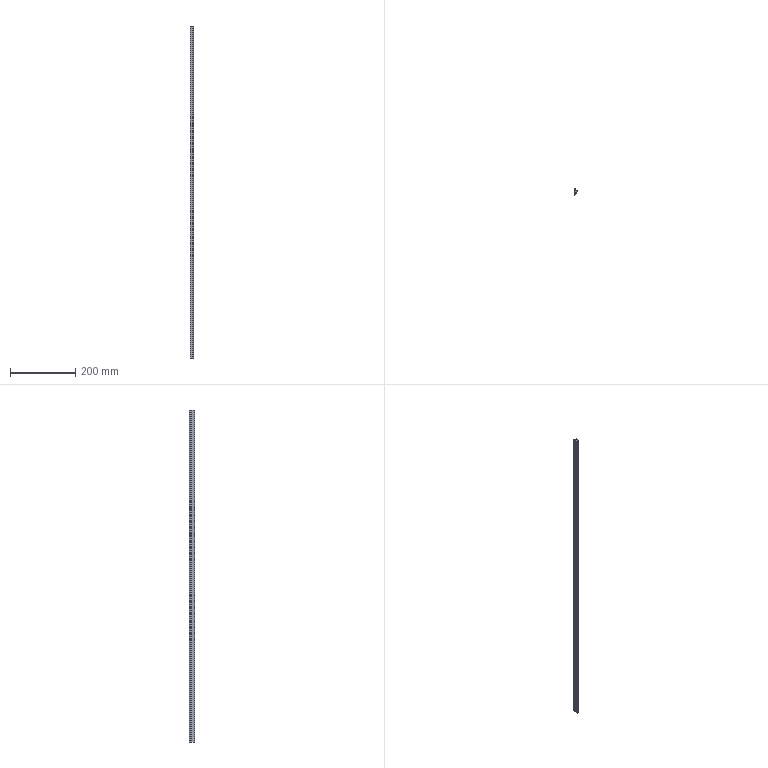Part | SolidWorks | features BaseBody 1, MoveFace 1 | 1 solid | 20 faces | box 10.8 x 17.5 x 1020 mm | volume 80377 mm3 | cylinder 11 | plane 9 | commonest cylinder face diameters 1.6 x2 14 x2 0.4 x1 0.6 x1 0.8 x1 2.6 x1
STEP:
#1=CARTESIAN_POINT('',(-3.236,-11.055,920.));
#2=VERTEX_POINT('',#1);
#3=CARTESIAN_POINT('',(-4.3,-10.3,920.));
#4=VERTEX_POINT('',#3);
#5=CARTESIAN_POINT('',(-3.5,-10.3,920.));
#6=DIRECTION('',(0.,0.,-1.));
#7=DIRECTION('',(1.,0.,0.));
#8=AXIS2_PLACEMENT_3D('',#5,#6,#7);
#9=CIRCLE('',#8,0.8);
#10=EDGE_CURVE('',#2,#4,#9,.T.);
#11=ORIENTED_EDGE('',*,*,#10,.T.);
#12=CARTESIAN_POINT('',(-4.3,-10.3,-100.));
#13=VERTEX_POINT('',#12);
#14=CARTESIAN_POINT('',(-4.3,-10.3,-100.));
#15=DIRECTION('',(0.,0.,-1.));
#16=VECTOR('',#15,1000.);
#17=LINE('',#14,#16);
#18=EDGE_CURVE('',#4,#13,#17,.T.);
#19=ORIENTED_EDGE('',*,*,#18,.T.);
#20=CARTESIAN_POINT('',(-3.236,-11.055,-100.));
#21=VERTEX_POINT('',#20);
#22=CARTESIAN_POINT('',(-3.5,-10.3,-100.));
#23=DIRECTION('',(0.,0.,1.));
#24=DIRECTION('',(-1.,0.,0.));
#25=AXIS2_PLACEMENT_3D('',#22,#23,#24);
#26=CIRCLE('',#25,0.8);
#27=EDGE_CURVE('',#13,#21,#26,.T.);
#28=ORIENTED_EDGE('',*,*,#27,.T.);
#29=CARTESIAN_POINT('',(-3.236,-11.055,-100.));
#30=DIRECTION('',(0.,0.,-1.));
#31=VECTOR('',#30,1000.);
#32=LINE('',#29,#31);
#33=EDGE_CURVE('',#2,#21,#32,.T.);
#34=ORIENTED_EDGE('',*,*,#33,.F.);
#35=EDGE_LOOP('',(#11,#19,#28,#34));
#36=FACE_OUTER_BOUND('',#35,.T.);
#37=CARTESIAN_POINT('',(-3.5,-10.3,-100.));
#38=DIRECTION('',(0.,0.,-1.));
#39=DIRECTION('',(-1.,0.,0.));
#40=AXIS2_PLACEMENT_3D('',#37,#38,#39);
#41=CYLINDRICAL_SURFACE('',#40,0.8);
#42=ADVANCED_FACE('',(#36),#41,.T.);
#43=CARTESIAN_POINT('',(1.184,-6.397,-100.));
#44=VERTEX_POINT('',#43);
#45=CARTESIAN_POINT('',(-5.702,-4.29,-100.));
#46=DIRECTION('',(0.,0.,1.));
#47=DIRECTION('',(-1.,0.,0.));
#48=AXIS2_PLACEMENT_3D('',#45,#46,#47);
#49=CIRCLE('',#48,7.201);
#50=EDGE_CURVE('',#21,#44,#49,.T.);
#51=ORIENTED_EDGE('',*,*,#50,.T.);
#52=CARTESIAN_POINT('',(1.184,-6.397,920.));
#53=VERTEX_POINT('',#52);
#54=CARTESIAN_POINT('',(1.184,-6.397,-100.));
#55=DIRECTION('',(0.,0.,1.));
#56=VECTOR('',#55,1000.);
#57=LINE('',#54,#56);
#58=EDGE_CURVE('',#44,#53,#57,.T.);
#59=ORIENTED_EDGE('',*,*,#58,.T.);
#60=CARTESIAN_POINT('',(-5.702,-4.29,920.));
#61=DIRECTION('',(0.,0.,-1.));
#62=DIRECTION('',(1.,0.,0.));
#63=AXIS2_PLACEMENT_3D('',#60,#61,#62);
#64=CIRCLE('',#63,7.201);
#65=EDGE_CURVE('',#53,#2,#64,.T.);
#66=ORIENTED_EDGE('',*,*,#65,.T.);
#67=ORIENTED_EDGE('',*,*,#33,.T.);
#68=EDGE_LOOP('',(#51,#59,#66,#67));
#69=FACE_OUTER_BOUND('',#68,.T.);
#70=CARTESIAN_POINT('',(-5.702,-4.29,-100.));
#71=DIRECTION('',(0.,0.,-1.));
#72=DIRECTION('',(-1.,0.,0.));
#73=AXIS2_PLACEMENT_3D('',#70,#71,#72);
#74=CYLINDRICAL_SURFACE('',#73,7.201);
#75=ADVANCED_FACE('',(#69),#74,.T.);
#76=CARTESIAN_POINT('',(0.9,-6.,-100.));
#77=VERTEX_POINT('',#76);
#78=CARTESIAN_POINT('',(0.9,-6.3,-100.));
#79=DIRECTION('',(0.,0.,1.));
#80=DIRECTION('',(-1.,0.,0.));
#81=AXIS2_PLACEMENT_3D('',#78,#79,#80);
#82=CIRCLE('',#81,0.3);
#83=EDGE_CURVE('',#44,#77,#82,.T.);
#84=ORIENTED_EDGE('',*,*,#83,.T.);
#85=CARTESIAN_POINT('',(0.9,-6.,920.));
#86=VERTEX_POINT('',#85);
#87=CARTESIAN_POINT('',(0.9,-6.,-100.));
#88=DIRECTION('',(0.,0.,1.));
#89=VECTOR('',#88,1000.);
#90=LINE('',#87,#89);
#91=EDGE_CURVE('',#77,#86,#90,.T.);
#92=ORIENTED_EDGE('',*,*,#91,.T.);
#93=CARTESIAN_POINT('',(0.9,-6.3,920.));
#94=DIRECTION('',(0.,0.,-1.));
#95=DIRECTION('',(1.,0.,0.));
#96=AXIS2_PLACEMENT_3D('',#93,#94,#95);
#97=CIRCLE('',#96,0.3);
#98=EDGE_CURVE('',#86,#53,#97,.T.);
#99=ORIENTED_EDGE('',*,*,#98,.T.);
#100=ORIENTED_EDGE('',*,*,#58,.F.);
#101=EDGE_LOOP('',(#84,#92,#99,#100));
#102=FACE_OUTER_BOUND('',#101,.T.);
#103=CARTESIAN_POINT('',(0.9,-6.3,-100.));
#104=DIRECTION('',(0.,0.,-1.));
#105=DIRECTION('',(-1.,0.,0.));
#106=AXIS2_PLACEMENT_3D('',#103,#104,#105);
#107=CYLINDRICAL_SURFACE('',#106,0.3);
#108=ADVANCED_FACE('',(#102),#107,.T.);
#109=CARTESIAN_POINT('',(-2.5,-0.5,-100.));
#110=VERTEX_POINT('',#109);
#111=CARTESIAN_POINT('',(-2.5,-6.153,-100.));
#112=VERTEX_POINT('',#111);
#113=CARTESIAN_POINT('',(-2.5,-6.397,-100.));
#114=DIRECTION('',(0.,-1.,0.));
#115=VECTOR('',#114,1000.);
#116=LINE('',#113,#115);
#117=EDGE_CURVE('',#110,#112,#116,.T.);
#118=ORIENTED_EDGE('',*,*,#117,.F.);
#119=CARTESIAN_POINT('',(-4.2,1.695,-100.));
#120=VERTEX_POINT('',#119);
#121=CARTESIAN_POINT('',(-1.701,1.875,-100.));
#122=DIRECTION('',(0.,0.,1.));
#123=DIRECTION('',(-1.,0.,0.));
#124=AXIS2_PLACEMENT_3D('',#121,#122,#123);
#125=CIRCLE('',#124,2.506);
#126=EDGE_CURVE('',#120,#110,#125,.T.);
#127=ORIENTED_EDGE('',*,*,#126,.F.);
#128=CARTESIAN_POINT('',(-4.2,5.1,-100.));
#129=VERTEX_POINT('',#128);
#130=CARTESIAN_POINT('',(-4.2,-6.397,-100.));
#131=DIRECTION('',(0.,-1.,0.));
#132=VECTOR('',#131,1000.);
#133=LINE('',#130,#132);
#134=EDGE_CURVE('',#129,#120,#133,.T.);
#135=ORIENTED_EDGE('',*,*,#134,.F.);
#136=CARTESIAN_POINT('',(-2.892,6.4,-100.));
#137=VERTEX_POINT('',#136);
#138=CARTESIAN_POINT('',(-2.9,5.1,-100.));
#139=DIRECTION('',(0.,0.,1.));
#140=DIRECTION('',(-1.,0.,0.));
#141=AXIS2_PLACEMENT_3D('',#138,#139,#140);
#142=CIRCLE('',#141,1.3);
#143=EDGE_CURVE('',#137,#129,#142,.T.);
#144=ORIENTED_EDGE('',*,*,#143,.F.);
#145=CARTESIAN_POINT('',(0.5,5.5,-100.));
#146=VERTEX_POINT('',#145);
#147=CARTESIAN_POINT('',(-2.934,-0.5999,-100.));
#148=DIRECTION('',(0.,0.,1.));
#149=DIRECTION('',(-1.,0.,0.));
#150=AXIS2_PLACEMENT_3D('',#147,#148,#149);
#151=CIRCLE('',#150,7.);
#152=EDGE_CURVE('',#146,#137,#151,.T.);
#153=ORIENTED_EDGE('',*,*,#152,.F.);
#154=CARTESIAN_POINT('',(5.5,1.7,-100.));
#155=VERTEX_POINT('',#154);
#156=CARTESIAN_POINT('',(5.5,1.7,-100.));
#157=DIRECTION('',(-0.7962,0.6051,0.));
#158=VECTOR('',#157,1000.);
#159=LINE('',#156,#158);
#160=EDGE_CURVE('',#155,#146,#159,.T.);
#161=ORIENTED_EDGE('',*,*,#160,.F.);
#162=CARTESIAN_POINT('',(6.458,-0.2215,-100.));
#163=VERTEX_POINT('',#162);
#164=CARTESIAN_POINT('',(6.458,-0.2215,-100.));
#165=DIRECTION('',(-0.4462,0.8949,0.));
#166=VECTOR('',#165,1000.);
#167=LINE('',#164,#166);
#168=EDGE_CURVE('',#163,#155,#167,.T.);
#169=ORIENTED_EDGE('',*,*,#168,.F.);
#170=CARTESIAN_POINT('',(5.895,-0.7433,-100.));
#171=VERTEX_POINT('',#170);
#172=CARTESIAN_POINT('',(6.1,-0.4,-100.));
#173=DIRECTION('',(0.,0.,1.));
#174=DIRECTION('',(-1.,0.,0.));
#175=AXIS2_PLACEMENT_3D('',#172,#173,#174);
#176=CIRCLE('',#175,0.4);
#177=EDGE_CURVE('',#171,#163,#176,.T.);
#178=ORIENTED_EDGE('',*,*,#177,.F.);
#179=CARTESIAN_POINT('',(3.,0.,-100.));
#180=VERTEX_POINT('',#179);
#181=CARTESIAN_POINT('',(2.746,-6.995,-100.));
#182=DIRECTION('',(0.,0.,-1.));
#183=DIRECTION('',(-1.,0.,0.));
#184=AXIS2_PLACEMENT_3D('',#181,#182,#183);
#185=CIRCLE('',#184,7.);
#186=EDGE_CURVE('',#180,#171,#185,.T.);
#187=ORIENTED_EDGE('',*,*,#186,.F.);
#188=CARTESIAN_POINT('',(0.,0.,-100.));
#189=VERTEX_POINT('',#188);
#190=CARTESIAN_POINT('',(-6.814,0.,-100.));
#191=DIRECTION('',(1.,0.,0.));
#192=VECTOR('',#191,1000.);
#193=LINE('',#190,#192);
#194=EDGE_CURVE('',#189,#180,#193,.T.);
#195=ORIENTED_EDGE('',*,*,#194,.F.);
#196=CARTESIAN_POINT('',(0.,-5.8,-100.));
#197=VERTEX_POINT('',#196);
#198=CARTESIAN_POINT('',(0.,-6.397,-100.));
#199=DIRECTION('',(0.,1.,0.));
#200=VECTOR('',#199,1000.);
#201=LINE('',#198,#200);
#202=EDGE_CURVE('',#197,#189,#201,.T.);
#203=ORIENTED_EDGE('',*,*,#202,.F.);
#204=CARTESIAN_POINT('',(0.2,-6.,-100.));
#205=VERTEX_POINT('',#204);
#206=CARTESIAN_POINT('',(0.2,-5.8,-100.));
#207=DIRECTION('',(0.,0.,1.));
#208=DIRECTION('',(-1.,0.,0.));
#209=AXIS2_PLACEMENT_3D('',#206,#207,#208);
#210=CIRCLE('',#209,0.2);
#211=EDGE_CURVE('',#197,#205,#210,.T.);
#212=ORIENTED_EDGE('',*,*,#211,.T.);
#213=CARTESIAN_POINT('',(-6.814,-6.,-100.));
#214=DIRECTION('',(-1.,0.,0.));
#215=VECTOR('',#214,1000.);
#216=LINE('',#213,#215);
#217=EDGE_CURVE('',#77,#205,#216,.T.);
#218=ORIENTED_EDGE('',*,*,#217,.F.);
#219=ORIENTED_EDGE('',*,*,#83,.F.);
#220=ORIENTED_EDGE('',*,*,#50,.F.);
#221=ORIENTED_EDGE('',*,*,#27,.F.);
#222=CARTESIAN_POINT('',(-3.998,-9.674,-100.));
#223=VERTEX_POINT('',#222);
#224=CARTESIAN_POINT('',(-3.5,-10.3,-100.));
#225=DIRECTION('',(0.,0.,1.));
#226=DIRECTION('',(-1.,0.,0.));
#227=AXIS2_PLACEMENT_3D('',#224,#225,#226);
#228=CIRCLE('',#227,0.8);
#229=EDGE_CURVE('',#223,#13,#228,.T.);
#230=ORIENTED_EDGE('',*,*,#229,.F.);
#231=CARTESIAN_POINT('',(-6.814,-6.397,-100.));
#232=DIRECTION('',(0.,0.,-1.));
#233=DIRECTION('',(-1.,0.,0.));
#234=AXIS2_PLACEMENT_3D('',#231,#232,#233);
#235=CIRCLE('',#234,4.321);
#236=EDGE_CURVE('',#112,#223,#235,.T.);
#237=ORIENTED_EDGE('',*,*,#236,.F.);
#238=EDGE_LOOP('',(#118,#127,#135,#144,#153,#161,#169,#178,#187,#195,#203,#212,#218,#219,#220,#221,#230,#237));
#239=FACE_OUTER_BOUND('',#238,.T.);
#240=CARTESIAN_POINT('',(-6.814,-6.397,-100.));
#241=DIRECTION('',(0.,0.,1.));
#242=DIRECTION('',(1.,0.,0.));
#243=AXIS2_PLACEMENT_3D('',#240,#241,#242);
#244=PLANE('',#243);
#245=ADVANCED_FACE('',(#239),#244,.F.);
#246=ORIENTED_EDGE('',*,*,#18,.F.);
#247=CARTESIAN_POINT('',(-3.998,-9.674,920.));
#248=VERTEX_POINT('',#247);
#249=CARTESIAN_POINT('',(-3.5,-10.3,920.));
#250=DIRECTION('',(0.,0.,-1.));
#251=DIRECTION('',(1.,0.,0.));
#252=AXIS2_PLACEMENT_3D('',#249,#250,#251);
#253=CIRCLE('',#252,0.8);
#254=EDGE_CURVE('',#4,#248,#253,.T.);
#255=ORIENTED_EDGE('',*,*,#254,.T.);
#256=CARTESIAN_POINT('',(-3.998,-9.674,-100.));
#257=DIRECTION('',(0.,0.,-1.));
#258=VECTOR('',#257,1000.);
#259=LINE('',#256,#258);
#260=EDGE_CURVE('',#248,#223,#259,.T.);
#261=ORIENTED_EDGE('',*,*,#260,.T.);
#262=ORIENTED_EDGE('',*,*,#229,.T.);
#263=EDGE_LOOP('',(#246,#255,#261,#262));
#264=FACE_OUTER_BOUND('',#263,.T.);
#265=CARTESIAN_POINT('',(-3.5,-10.3,-100.));
#266=DIRECTION('',(0.,0.,-1.));
#267=DIRECTION('',(-1.,0.,0.));
#268=AXIS2_PLACEMENT_3D('',#265,#266,#267);
#269=CYLINDRICAL_SURFACE('',#268,0.8);
#270=ADVANCED_FACE('',(#264),#269,.T.);
#271=CARTESIAN_POINT('',(-4.2,1.695,920.));
#272=VERTEX_POINT('',#271);
#273=CARTESIAN_POINT('',(-2.5,-0.5,920.));
#274=VERTEX_POINT('',#273);
#275=CARTESIAN_POINT('',(-1.701,1.875,920.));
#276=DIRECTION('',(0.,0.,1.));
#277=DIRECTION('',(1.,0.,0.));
#278=AXIS2_PLACEMENT_3D('',#275,#276,#277);
#279=CIRCLE('',#278,2.506);
#280=EDGE_CURVE('',#272,#274,#279,.T.);
#281=ORIENTED_EDGE('',*,*,#280,.T.);
#282=CARTESIAN_POINT('',(-2.5,-6.153,920.));
#283=VERTEX_POINT('',#282);
#284=CARTESIAN_POINT('',(-2.5,-6.397,920.));
#285=DIRECTION('',(0.,-1.,0.));
#286=VECTOR('',#285,1000.);
#287=LINE('',#284,#286);
#288=EDGE_CURVE('',#274,#283,#287,.T.);
#289=ORIENTED_EDGE('',*,*,#288,.T.);
#290=CARTESIAN_POINT('',(-6.814,-6.397,920.));
#291=DIRECTION('',(0.,0.,-1.));
#292=DIRECTION('',(1.,0.,0.));
#293=AXIS2_PLACEMENT_3D('',#290,#291,#292);
#294=CIRCLE('',#293,4.321);
#295=EDGE_CURVE('',#283,#248,#294,.T.);
#296=ORIENTED_EDGE('',*,*,#295,.T.);
#297=ORIENTED_EDGE('',*,*,#254,.F.);
#298=ORIENTED_EDGE('',*,*,#10,.F.);
#299=ORIENTED_EDGE('',*,*,#65,.F.);
#300=ORIENTED_EDGE('',*,*,#98,.F.);
#301=CARTESIAN_POINT('',(0.2,-6.,920.));
#302=VERTEX_POINT('',#301);
#303=CARTESIAN_POINT('',(-6.814,-6.,920.));
#304=DIRECTION('',(-1.,0.,0.));
#305=VECTOR('',#304,1000.);
#306=LINE('',#303,#305);
#307=EDGE_CURVE('',#86,#302,#306,.T.);
#308=ORIENTED_EDGE('',*,*,#307,.T.);
#309=CARTESIAN_POINT('',(0.,-5.8,920.));
#310=VERTEX_POINT('',#309);
#311=CARTESIAN_POINT('',(0.2,-5.8,920.));
#312=DIRECTION('',(0.,0.,-1.));
#313=DIRECTION('',(1.,0.,0.));
#314=AXIS2_PLACEMENT_3D('',#311,#312,#313);
#315=CIRCLE('',#314,0.2);
#316=EDGE_CURVE('',#302,#310,#315,.T.);
#317=ORIENTED_EDGE('',*,*,#316,.T.);
#318=CARTESIAN_POINT('',(0.,0.,920.));
#319=VERTEX_POINT('',#318);
#320=CARTESIAN_POINT('',(0.,-6.397,920.));
#321=DIRECTION('',(0.,1.,0.));
#322=VECTOR('',#321,1000.);
#323=LINE('',#320,#322);
#324=EDGE_CURVE('',#310,#319,#323,.T.);
#325=ORIENTED_EDGE('',*,*,#324,.T.);
#326=CARTESIAN_POINT('',(3.,0.,920.));
#327=VERTEX_POINT('',#326);
#328=CARTESIAN_POINT('',(-6.814,0.,920.));
#329=DIRECTION('',(1.,0.,0.));
#330=VECTOR('',#329,1000.);
#331=LINE('',#328,#330);
#332=EDGE_CURVE('',#319,#327,#331,.T.);
#333=ORIENTED_EDGE('',*,*,#332,.T.);
#334=CARTESIAN_POINT('',(5.895,-0.7433,920.));
#335=VERTEX_POINT('',#334);
#336=CARTESIAN_POINT('',(2.746,-6.995,920.));
#337=DIRECTION('',(0.,0.,-1.));
#338=DIRECTION('',(1.,0.,0.));
#339=AXIS2_PLACEMENT_3D('',#336,#337,#338);
#340=CIRCLE('',#339,7.);
#341=EDGE_CURVE('',#327,#335,#340,.T.);
#342=ORIENTED_EDGE('',*,*,#341,.T.);
#343=CARTESIAN_POINT('',(6.458,-0.2215,920.));
#344=VERTEX_POINT('',#343);
#345=CARTESIAN_POINT('',(6.1,-0.4,920.));
#346=DIRECTION('',(0.,0.,-1.));
#347=DIRECTION('',(1.,0.,0.));
#348=AXIS2_PLACEMENT_3D('',#345,#346,#347);
#349=CIRCLE('',#348,0.4);
#350=EDGE_CURVE('',#344,#335,#349,.T.);
#351=ORIENTED_EDGE('',*,*,#350,.F.);
#352=CARTESIAN_POINT('',(5.5,1.7,920.));
#353=VERTEX_POINT('',#352);
#354=CARTESIAN_POINT('',(6.282,0.1323,920.));
#355=DIRECTION('',(-0.4462,0.8949,0.));
#356=VECTOR('',#355,1000.);
#357=LINE('',#354,#356);
#358=EDGE_CURVE('',#344,#353,#357,.T.);
#359=ORIENTED_EDGE('',*,*,#358,.T.);
#360=CARTESIAN_POINT('',(0.5,5.5,920.));
#361=VERTEX_POINT('',#360);
#362=CARTESIAN_POINT('',(1.595,4.668,920.));
#363=DIRECTION('',(-0.7962,0.6051,0.));
#364=VECTOR('',#363,1000.);
#365=LINE('',#362,#364);
#366=EDGE_CURVE('',#353,#361,#365,.T.);
#367=ORIENTED_EDGE('',*,*,#366,.T.);
#368=CARTESIAN_POINT('',(-2.892,6.4,920.));
#369=VERTEX_POINT('',#368);
#370=CARTESIAN_POINT('',(-2.934,-0.5999,920.));
#371=DIRECTION('',(0.,0.,1.));
#372=DIRECTION('',(1.,0.,0.));
#373=AXIS2_PLACEMENT_3D('',#370,#371,#372);
#374=CIRCLE('',#373,7.);
#375=EDGE_CURVE('',#361,#369,#374,.T.);
#376=ORIENTED_EDGE('',*,*,#375,.T.);
#377=CARTESIAN_POINT('',(-4.2,5.1,920.));
#378=VERTEX_POINT('',#377);
#379=CARTESIAN_POINT('',(-2.9,5.1,920.));
#380=DIRECTION('',(0.,0.,1.));
#381=DIRECTION('',(1.,0.,0.));
#382=AXIS2_PLACEMENT_3D('',#379,#380,#381);
#383=CIRCLE('',#382,1.3);
#384=EDGE_CURVE('',#369,#378,#383,.T.);
#385=ORIENTED_EDGE('',*,*,#384,.T.);
#386=CARTESIAN_POINT('',(-4.2,-6.397,920.));
#387=DIRECTION('',(0.,-1.,0.));
#388=VECTOR('',#387,1000.);
#389=LINE('',#386,#388);
#390=EDGE_CURVE('',#378,#272,#389,.T.);
#391=ORIENTED_EDGE('',*,*,#390,.T.);
#392=EDGE_LOOP('',(#281,#289,#296,#297,#298,#299,#300,#308,#317,#325,#333,#342,#351,#359,#367,#376,#385,#391));
#393=FACE_OUTER_BOUND('',#392,.T.);
#394=CARTESIAN_POINT('',(-6.814,-6.397,920.));
#395=DIRECTION('',(0.,0.,1.));
#396=DIRECTION('',(1.,0.,0.));
#397=AXIS2_PLACEMENT_3D('',#394,#395,#396);
#398=PLANE('',#397);
#399=ADVANCED_FACE('',(#393),#398,.T.);
#400=ORIENTED_EDGE('',*,*,#217,.T.);
#401=CARTESIAN_POINT('',(0.2,-6.,-100.));
#402=DIRECTION('',(0.,0.,1.));
#403=VECTOR('',#402,1000.);
#404=LINE('',#401,#403);
#405=EDGE_CURVE('',#205,#302,#404,.T.);
#406=ORIENTED_EDGE('',*,*,#405,.T.);
#407=ORIENTED_EDGE('',*,*,#307,.F.);
#408=ORIENTED_EDGE('',*,*,#91,.F.);
#409=EDGE_LOOP('',(#400,#406,#407,#408));
#410=FACE_OUTER_BOUND('',#409,.T.);
#411=CARTESIAN_POINT('',(0.9,-6.,-100.));
#412=DIRECTION('',(0.,1.,0.));
#413=DIRECTION('',(0.,0.,1.));
#414=AXIS2_PLACEMENT_3D('',#411,#412,#413);
#415=PLANE('',#414);
#416=ADVANCED_FACE('',(#410),#415,.T.);
#417=CARTESIAN_POINT('',(-2.5,-6.153,-100.));
#418=DIRECTION('',(0.,0.,1.));
#419=VECTOR('',#418,1000.);
#420=LINE('',#417,#419);
#421=EDGE_CURVE('',#112,#283,#420,.T.);
#422=ORIENTED_EDGE('',*,*,#421,.F.);
#423=ORIENTED_EDGE('',*,*,#236,.T.);
#424=ORIENTED_EDGE('',*,*,#260,.F.);
#425=ORIENTED_EDGE('',*,*,#295,.F.);
#426=EDGE_LOOP('',(#422,#423,#424,#425));
#427=FACE_OUTER_BOUND('',#426,.T.);
#428=CARTESIAN_POINT('',(-6.814,-6.397,-100.));
#429=DIRECTION('',(0.,0.,-1.));
#430=DIRECTION('',(-1.,0.,0.));
#431=AXIS2_PLACEMENT_3D('',#428,#429,#430);
#432=CYLINDRICAL_SURFACE('',#431,4.321);
#433=ADVANCED_FACE('',(#427),#432,.F.);
#434=ORIENTED_EDGE('',*,*,#117,.T.);
#435=ORIENTED_EDGE('',*,*,#421,.T.);
#436=ORIENTED_EDGE('',*,*,#288,.F.);
#437=CARTESIAN_POINT('',(-2.5,-0.5,-100.));
#438=DIRECTION('',(0.,0.,-1.));
#439=VECTOR('',#438,1000.);
#440=LINE('',#437,#439);
#441=EDGE_CURVE('',#274,#110,#440,.T.);
#442=ORIENTED_EDGE('',*,*,#441,.T.);
#443=EDGE_LOOP('',(#434,#435,#436,#442));
#444=FACE_OUTER_BOUND('',#443,.T.);
#445=CARTESIAN_POINT('',(-2.5,-0.5,-100.));
#446=DIRECTION('',(-1.,0.,0.));
#447=DIRECTION('',(0.,0.,1.));
#448=AXIS2_PLACEMENT_3D('',#445,#446,#447);
#449=PLANE('',#448);
#450=ADVANCED_FACE('',(#444),#449,.T.);
#451=ORIENTED_EDGE('',*,*,#126,.T.);
#452=ORIENTED_EDGE('',*,*,#441,.F.);
#453=ORIENTED_EDGE('',*,*,#280,.F.);
#454=CARTESIAN_POINT('',(-4.2,1.695,-100.));
#455=DIRECTION('',(0.,0.,-1.));
#456=VECTOR('',#455,1000.);
#457=LINE('',#454,#456);
#458=EDGE_CURVE('',#272,#120,#457,.T.);
#459=ORIENTED_EDGE('',*,*,#458,.T.);
#460=EDGE_LOOP('',(#451,#452,#453,#459));
#461=FACE_OUTER_BOUND('',#460,.T.);
#462=CARTESIAN_POINT('',(-1.701,1.875,-100.));
#463=DIRECTION('',(0.,0.,-1.));
#464=DIRECTION('',(-1.,0.,0.));
#465=AXIS2_PLACEMENT_3D('',#462,#463,#464);
#466=CYLINDRICAL_SURFACE('',#465,2.506);
#467=ADVANCED_FACE('',(#461),#466,.T.);
#468=ORIENTED_EDGE('',*,*,#134,.T.);
#469=ORIENTED_EDGE('',*,*,#458,.F.);
#470=ORIENTED_EDGE('',*,*,#390,.F.);
#471=CARTESIAN_POINT('',(-4.2,5.1,-100.));
#472=DIRECTION('',(0.,0.,-1.));
#473=VECTOR('',#472,1000.);
#474=LINE('',#471,#473);
#475=EDGE_CURVE('',#378,#129,#474,.T.);
#476=ORIENTED_EDGE('',*,*,#475,.T.);
#477=EDGE_LOOP('',(#468,#469,#470,#476));
#478=FACE_OUTER_BOUND('',#477,.T.);
#479=CARTESIAN_POINT('',(-4.2,5.1,-100.));
#480=DIRECTION('',(-1.,0.,0.));
#481=DIRECTION('',(0.,0.,1.));
#482=AXIS2_PLACEMENT_3D('',#479,#480,#481);
#483=PLANE('',#482);
#484=ADVANCED_FACE('',(#478),#483,.T.);
#485=ORIENTED_EDGE('',*,*,#143,.T.);
#486=ORIENTED_EDGE('',*,*,#475,.F.);
#487=ORIENTED_EDGE('',*,*,#384,.F.);
#488=CARTESIAN_POINT('',(-2.892,6.4,-100.));
#489=DIRECTION('',(0.,0.,-1.));
#490=VECTOR('',#489,1000.);
#491=LINE('',#488,#490);
#492=EDGE_CURVE('',#369,#137,#491,.T.);
#493=ORIENTED_EDGE('',*,*,#492,.T.);
#494=EDGE_LOOP('',(#485,#486,#487,#493));
#495=FACE_OUTER_BOUND('',#494,.T.);
#496=CARTESIAN_POINT('',(-2.9,5.1,-100.));
#497=DIRECTION('',(0.,0.,-1.));
#498=DIRECTION('',(-1.,0.,0.));
#499=AXIS2_PLACEMENT_3D('',#496,#497,#498);
#500=CYLINDRICAL_SURFACE('',#499,1.3);
#501=ADVANCED_FACE('',(#495),#500,.T.);
#502=ORIENTED_EDGE('',*,*,#152,.T.);
#503=ORIENTED_EDGE('',*,*,#492,.F.);
#504=ORIENTED_EDGE('',*,*,#375,.F.);
#505=CARTESIAN_POINT('',(0.5,5.5,-100.));
#506=DIRECTION('',(0.,0.,-1.));
#507=VECTOR('',#506,1000.);
#508=LINE('',#505,#507);
#509=EDGE_CURVE('',#361,#146,#508,.T.);
#510=ORIENTED_EDGE('',*,*,#509,.T.);
#511=EDGE_LOOP('',(#502,#503,#504,#510));
#512=FACE_OUTER_BOUND('',#511,.T.);
#513=CARTESIAN_POINT('',(-2.934,-0.5999,-100.));
#514=DIRECTION('',(0.,0.,-1.));
#515=DIRECTION('',(-1.,0.,0.));
#516=AXIS2_PLACEMENT_3D('',#513,#514,#515);
#517=CYLINDRICAL_SURFACE('',#516,7.);
#518=ADVANCED_FACE('',(#512),#517,.T.);
#519=ORIENTED_EDGE('',*,*,#160,.T.);
#520=ORIENTED_EDGE('',*,*,#509,.F.);
#521=ORIENTED_EDGE('',*,*,#366,.F.);
#522=CARTESIAN_POINT('',(5.5,1.7,-100.));
#523=DIRECTION('',(0.,0.,-1.));
#524=VECTOR('',#523,1000.);
#525=LINE('',#522,#524);
#526=EDGE_CURVE('',#353,#155,#525,.T.);
#527=ORIENTED_EDGE('',*,*,#526,.T.);
#528=EDGE_LOOP('',(#519,#520,#521,#527));
#529=FACE_OUTER_BOUND('',#528,.T.);
#530=CARTESIAN_POINT('',(5.5,1.7,-100.));
#531=DIRECTION('',(0.6051,0.7962,0.));
#532=DIRECTION('',(-0.7962,0.6051,0.));
#533=AXIS2_PLACEMENT_3D('',#530,#531,#532);
#534=PLANE('',#533);
#535=ADVANCED_FACE('',(#529),#534,.T.);
#536=ORIENTED_EDGE('',*,*,#168,.T.);
#537=ORIENTED_EDGE('',*,*,#526,.F.);
#538=ORIENTED_EDGE('',*,*,#358,.F.);
#539=CARTESIAN_POINT('',(6.458,-0.2215,-100.));
#540=DIRECTION('',(0.,0.,-1.));
#541=VECTOR('',#540,1000.);
#542=LINE('',#539,#541);
#543=EDGE_CURVE('',#344,#163,#542,.T.);
#544=ORIENTED_EDGE('',*,*,#543,.T.);
#545=EDGE_LOOP('',(#536,#537,#538,#544));
#546=FACE_OUTER_BOUND('',#545,.T.);
#547=CARTESIAN_POINT('',(6.458,-0.2215,-100.));
#548=DIRECTION('',(0.8949,0.4462,0.));
#549=DIRECTION('',(-0.4462,0.8949,0.));
#550=AXIS2_PLACEMENT_3D('',#547,#548,#549);
#551=PLANE('',#550);
#552=ADVANCED_FACE('',(#546),#551,.T.);
#553=CARTESIAN_POINT('',(3.,0.,-100.));
#554=DIRECTION('',(0.,0.,1.));
#555=VECTOR('',#554,1000.);
#556=LINE('',#553,#555);
#557=EDGE_CURVE('',#180,#327,#556,.T.);
#558=ORIENTED_EDGE('',*,*,#557,.F.);
#559=ORIENTED_EDGE('',*,*,#186,.T.);
#560=CARTESIAN_POINT('',(5.895,-0.7433,-100.));
#561=DIRECTION('',(0.,0.,-1.));
#562=VECTOR('',#561,1000.);
#563=LINE('',#560,#562);
#564=EDGE_CURVE('',#335,#171,#563,.T.);
#565=ORIENTED_EDGE('',*,*,#564,.F.);
#566=ORIENTED_EDGE('',*,*,#341,.F.);
#567=EDGE_LOOP('',(#558,#559,#565,#566));
#568=FACE_OUTER_BOUND('',#567,.T.);
#569=CARTESIAN_POINT('',(2.746,-6.995,-100.));
#570=DIRECTION('',(0.,0.,-1.));
#571=DIRECTION('',(-1.,0.,0.));
#572=AXIS2_PLACEMENT_3D('',#569,#570,#571);
#573=CYLINDRICAL_SURFACE('',#572,7.);
#574=ADVANCED_FACE('',(#568),#573,.F.);
#575=ORIENTED_EDGE('',*,*,#194,.T.);
#576=ORIENTED_EDGE('',*,*,#557,.T.);
#577=ORIENTED_EDGE('',*,*,#332,.F.);
#578=CARTESIAN_POINT('',(0.,0.,-100.));
#579=DIRECTION('',(0.,0.,-1.));
#580=VECTOR('',#579,1000.);
#581=LINE('',#578,#580);
#582=EDGE_CURVE('',#319,#189,#581,.T.);
#583=ORIENTED_EDGE('',*,*,#582,.T.);
#584=EDGE_LOOP('',(#575,#576,#577,#583));
#585=FACE_OUTER_BOUND('',#584,.T.);
#586=CARTESIAN_POINT('',(0.,0.,-100.));
#587=DIRECTION('',(0.,-1.,0.));
#588=DIRECTION('',(0.,0.,-1.));
#589=AXIS2_PLACEMENT_3D('',#586,#587,#588);
#590=PLANE('',#589);
#591=ADVANCED_FACE('',(#585),#590,.T.);
#592=ORIENTED_EDGE('',*,*,#202,.T.);
#593=ORIENTED_EDGE('',*,*,#582,.F.);
#594=ORIENTED_EDGE('',*,*,#324,.F.);
#595=CARTESIAN_POINT('',(0.,-5.8,-100.));
#596=DIRECTION('',(0.,0.,-1.));
#597=VECTOR('',#596,1000.);
#598=LINE('',#595,#597);
#599=EDGE_CURVE('',#310,#197,#598,.T.);
#600=ORIENTED_EDGE('',*,*,#599,.T.);
#601=EDGE_LOOP('',(#592,#593,#594,#600));
#602=FACE_OUTER_BOUND('',#601,.T.);
#603=CARTESIAN_POINT('',(0.,-5.8,-100.));
#604=DIRECTION('',(1.,0.,0.));
#605=DIRECTION('',(0.,0.,-1.));
#606=AXIS2_PLACEMENT_3D('',#603,#604,#605);
#607=PLANE('',#606);
#608=ADVANCED_FACE('',(#602),#607,.T.);
#609=ORIENTED_EDGE('',*,*,#405,.F.);
#610=ORIENTED_EDGE('',*,*,#211,.F.);
#611=ORIENTED_EDGE('',*,*,#599,.F.);
#612=ORIENTED_EDGE('',*,*,#316,.F.);
#613=EDGE_LOOP('',(#609,#610,#611,#612));
#614=FACE_OUTER_BOUND('',#613,.T.);
#615=CARTESIAN_POINT('',(0.2,-5.8,-100.));
#616=DIRECTION('',(0.,0.,-1.));
#617=DIRECTION('',(-1.,0.,0.));
#618=AXIS2_PLACEMENT_3D('',#615,#616,#617);
#619=CYLINDRICAL_SURFACE('',#618,0.2);
#620=ADVANCED_FACE('',(#614),#619,.F.);
#621=ORIENTED_EDGE('',*,*,#177,.T.);
#622=ORIENTED_EDGE('',*,*,#543,.F.);
#623=ORIENTED_EDGE('',*,*,#350,.T.);
#624=ORIENTED_EDGE('',*,*,#564,.T.);
#625=EDGE_LOOP('',(#621,#622,#623,#624));
#626=FACE_OUTER_BOUND('',#625,.T.);
#627=CARTESIAN_POINT('',(6.1,-0.4,-100.));
#628=DIRECTION('',(0.,0.,-1.));
#629=DIRECTION('',(-1.,0.,0.));
#630=AXIS2_PLACEMENT_3D('',#627,#628,#629);
#631=CYLINDRICAL_SURFACE('',#630,0.4);
#632=ADVANCED_FACE('',(#626),#631,.T.);
#633=CLOSED_SHELL('',(#42,#75,#108,#245,#270,#399,#416,#433,#450,#467,#484,#501,#518,#535,#552,#574,#591,#608,#620,#632));
#634=MANIFOLD_SOLID_BREP('',#633);
#635=CARTESIAN_POINT('',(0.,0.,0.));
#636=DIRECTION('',(0.,0.,1.));
#637=DIRECTION('',(1.,0.,0.));
#638=AXIS2_PLACEMENT_3D('',#635,#636,#637);
#639=(LENGTH_UNIT()NAMED_UNIT(*)SI_UNIT(.MILLI.,.METRE.));
#640=UNCERTAINTY_MEASURE_WITH_UNIT(LENGTH_MEASURE(0.00001),#639,'','');
#641=(NAMED_UNIT(*)PLANE_ANGLE_UNIT()SI_UNIT($,.RADIAN.));
#642=(NAMED_UNIT(*)SI_UNIT($,.STERADIAN.)SOLID_ANGLE_UNIT());
#643=(GEOMETRIC_REPRESENTATION_CONTEXT(3)GLOBAL_UNCERTAINTY_ASSIGNED_CONTEXT((#640))GLOBAL_UNIT_ASSIGNED_CONTEXT((#639,#641,#642))REPRESENTATION_CONTEXT('',''));
#644=ADVANCED_BREP_SHAPE_REPRESENTATION('',(#634,#638),#643);